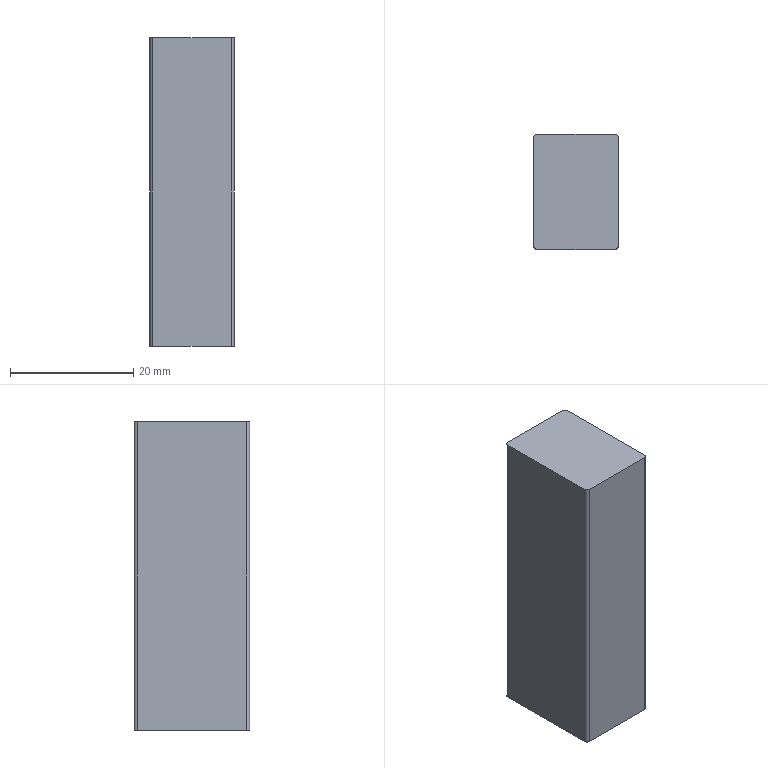Part | NX | features BREP 1 | 1 solid | 10 faces | box 13.656 x 18.683 x 50 mm | volume 12746 mm3 | plane 6 | cylinder 4 | commonest cylinder face diameters 1 x4
STEP:
#1=CARTESIAN_POINT('',(-6.328,9.342,-40.6));
#2=VERTEX_POINT('',#1);
#3=CARTESIAN_POINT('',(-6.828,8.842,-40.6));
#4=VERTEX_POINT('',#3);
#5=CARTESIAN_POINT('',(-6.328,8.842,-40.6));
#6=DIRECTION('',(0.,0.,1.));
#7=DIRECTION('',(1.,0.,0.));
#8=AXIS2_PLACEMENT_3D('',#5,#6,#7);
#9=CIRCLE('',#8,0.5);
#10=EDGE_CURVE('',#2,#4,#9,.T.);
#11=ORIENTED_EDGE('',*,*,#10,.F.);
#12=CARTESIAN_POINT('',(-6.328,9.342,-90.6));
#13=VERTEX_POINT('',#12);
#14=CARTESIAN_POINT('',(-6.328,9.342,-90.6));
#15=DIRECTION('',(0.,0.,1.));
#16=VECTOR('',#15,1000.);
#17=LINE('',#14,#16);
#18=EDGE_CURVE('',#13,#2,#17,.T.);
#19=ORIENTED_EDGE('',*,*,#18,.F.);
#20=CARTESIAN_POINT('',(-6.828,8.842,-90.6));
#21=VERTEX_POINT('',#20);
#22=CARTESIAN_POINT('',(-6.328,8.842,-90.6));
#23=DIRECTION('',(0.,0.,1.));
#24=DIRECTION('',(1.,0.,0.));
#25=AXIS2_PLACEMENT_3D('',#22,#23,#24);
#26=CIRCLE('',#25,0.5);
#27=EDGE_CURVE('',#13,#21,#26,.T.);
#28=ORIENTED_EDGE('',*,*,#27,.T.);
#29=CARTESIAN_POINT('',(-6.828,8.842,-90.6));
#30=DIRECTION('',(0.,0.,1.));
#31=VECTOR('',#30,1000.);
#32=LINE('',#29,#31);
#33=EDGE_CURVE('',#21,#4,#32,.T.);
#34=ORIENTED_EDGE('',*,*,#33,.T.);
#35=EDGE_LOOP('',(#11,#19,#28,#34));
#36=FACE_BOUND('',#35,.T.);
#37=CARTESIAN_POINT('',(-6.328,8.842,-90.6));
#38=DIRECTION('',(0.,0.,1.));
#39=DIRECTION('',(-1.,0.,0.));
#40=AXIS2_PLACEMENT_3D('',#37,#38,#39);
#41=CYLINDRICAL_SURFACE('',#40,0.5);
#42=ADVANCED_FACE('',(#36),#41,.T.);
#43=CARTESIAN_POINT('',(-6.828,-8.842,-40.6));
#44=VERTEX_POINT('',#43);
#45=CARTESIAN_POINT('',(-6.828,-8.842,-40.6));
#46=DIRECTION('',(0.,1.,0.));
#47=VECTOR('',#46,1000.);
#48=LINE('',#45,#47);
#49=EDGE_CURVE('',#44,#4,#48,.T.);
#50=ORIENTED_EDGE('',*,*,#49,.T.);
#51=ORIENTED_EDGE('',*,*,#33,.F.);
#52=CARTESIAN_POINT('',(-6.828,-8.842,-90.6));
#53=VERTEX_POINT('',#52);
#54=CARTESIAN_POINT('',(-6.828,-8.842,-90.6));
#55=DIRECTION('',(0.,1.,0.));
#56=VECTOR('',#55,1000.);
#57=LINE('',#54,#56);
#58=EDGE_CURVE('',#53,#21,#57,.T.);
#59=ORIENTED_EDGE('',*,*,#58,.F.);
#60=CARTESIAN_POINT('',(-6.828,-8.842,-90.6));
#61=DIRECTION('',(0.,0.,1.));
#62=VECTOR('',#61,1000.);
#63=LINE('',#60,#62);
#64=EDGE_CURVE('',#53,#44,#63,.T.);
#65=ORIENTED_EDGE('',*,*,#64,.T.);
#66=EDGE_LOOP('',(#50,#51,#59,#65));
#67=FACE_BOUND('',#66,.T.);
#68=CARTESIAN_POINT('',(-6.828,-8.842,-90.6));
#69=DIRECTION('',(1.,0.,0.));
#70=DIRECTION('',(0.,-1.,0.));
#71=AXIS2_PLACEMENT_3D('',#68,#69,#70);
#72=PLANE('',#71);
#73=ADVANCED_FACE('',(#67),#72,.F.);
#74=CARTESIAN_POINT('',(-6.328,-9.342,-40.6));
#75=VERTEX_POINT('',#74);
#76=CARTESIAN_POINT('',(-6.328,-8.842,-40.6));
#77=DIRECTION('',(0.,0.,1.));
#78=DIRECTION('',(1.,0.,0.));
#79=AXIS2_PLACEMENT_3D('',#76,#77,#78);
#80=CIRCLE('',#79,0.5);
#81=EDGE_CURVE('',#44,#75,#80,.T.);
#82=ORIENTED_EDGE('',*,*,#81,.F.);
#83=ORIENTED_EDGE('',*,*,#64,.F.);
#84=CARTESIAN_POINT('',(-6.328,-9.342,-90.6));
#85=VERTEX_POINT('',#84);
#86=CARTESIAN_POINT('',(-6.328,-8.842,-90.6));
#87=DIRECTION('',(0.,0.,1.));
#88=DIRECTION('',(1.,0.,0.));
#89=AXIS2_PLACEMENT_3D('',#86,#87,#88);
#90=CIRCLE('',#89,0.5);
#91=EDGE_CURVE('',#53,#85,#90,.T.);
#92=ORIENTED_EDGE('',*,*,#91,.T.);
#93=CARTESIAN_POINT('',(-6.328,-9.342,-90.6));
#94=DIRECTION('',(0.,0.,1.));
#95=VECTOR('',#94,1000.);
#96=LINE('',#93,#95);
#97=EDGE_CURVE('',#85,#75,#96,.T.);
#98=ORIENTED_EDGE('',*,*,#97,.T.);
#99=EDGE_LOOP('',(#82,#83,#92,#98));
#100=FACE_BOUND('',#99,.T.);
#101=CARTESIAN_POINT('',(-6.328,-8.842,-90.6));
#102=DIRECTION('',(0.,0.,1.));
#103=DIRECTION('',(-1.,0.,0.));
#104=AXIS2_PLACEMENT_3D('',#101,#102,#103);
#105=CYLINDRICAL_SURFACE('',#104,0.5);
#106=ADVANCED_FACE('',(#100),#105,.T.);
#107=CARTESIAN_POINT('',(6.328,-9.342,-40.6));
#108=VERTEX_POINT('',#107);
#109=CARTESIAN_POINT('',(6.328,-9.342,-40.6));
#110=DIRECTION('',(-1.,0.,0.));
#111=VECTOR('',#110,1000.);
#112=LINE('',#109,#111);
#113=EDGE_CURVE('',#108,#75,#112,.T.);
#114=ORIENTED_EDGE('',*,*,#113,.T.);
#115=ORIENTED_EDGE('',*,*,#97,.F.);
#116=CARTESIAN_POINT('',(6.328,-9.342,-90.6));
#117=VERTEX_POINT('',#116);
#118=CARTESIAN_POINT('',(6.328,-9.342,-90.6));
#119=DIRECTION('',(-1.,0.,0.));
#120=VECTOR('',#119,1000.);
#121=LINE('',#118,#120);
#122=EDGE_CURVE('',#117,#85,#121,.T.);
#123=ORIENTED_EDGE('',*,*,#122,.F.);
#124=CARTESIAN_POINT('',(6.328,-9.342,-90.6));
#125=DIRECTION('',(0.,0.,1.));
#126=VECTOR('',#125,1000.);
#127=LINE('',#124,#126);
#128=EDGE_CURVE('',#117,#108,#127,.T.);
#129=ORIENTED_EDGE('',*,*,#128,.T.);
#130=EDGE_LOOP('',(#114,#115,#123,#129));
#131=FACE_BOUND('',#130,.T.);
#132=CARTESIAN_POINT('',(6.328,-9.342,-90.6));
#133=DIRECTION('',(0.,1.,0.));
#134=DIRECTION('',(0.,0.,-1.));
#135=AXIS2_PLACEMENT_3D('',#132,#133,#134);
#136=PLANE('',#135);
#137=ADVANCED_FACE('',(#131),#136,.F.);
#138=CARTESIAN_POINT('',(6.828,-8.842,-40.6));
#139=VERTEX_POINT('',#138);
#140=CARTESIAN_POINT('',(6.328,-8.842,-40.6));
#141=DIRECTION('',(0.,0.,1.));
#142=DIRECTION('',(1.,0.,0.));
#143=AXIS2_PLACEMENT_3D('',#140,#141,#142);
#144=CIRCLE('',#143,0.5);
#145=EDGE_CURVE('',#108,#139,#144,.T.);
#146=ORIENTED_EDGE('',*,*,#145,.F.);
#147=ORIENTED_EDGE('',*,*,#128,.F.);
#148=CARTESIAN_POINT('',(6.828,-8.842,-90.6));
#149=VERTEX_POINT('',#148);
#150=CARTESIAN_POINT('',(6.328,-8.842,-90.6));
#151=DIRECTION('',(0.,0.,1.));
#152=DIRECTION('',(1.,0.,0.));
#153=AXIS2_PLACEMENT_3D('',#150,#151,#152);
#154=CIRCLE('',#153,0.5);
#155=EDGE_CURVE('',#117,#149,#154,.T.);
#156=ORIENTED_EDGE('',*,*,#155,.T.);
#157=CARTESIAN_POINT('',(6.828,-8.842,-90.6));
#158=DIRECTION('',(0.,0.,1.));
#159=VECTOR('',#158,1000.);
#160=LINE('',#157,#159);
#161=EDGE_CURVE('',#149,#139,#160,.T.);
#162=ORIENTED_EDGE('',*,*,#161,.T.);
#163=EDGE_LOOP('',(#146,#147,#156,#162));
#164=FACE_BOUND('',#163,.T.);
#165=CARTESIAN_POINT('',(6.328,-8.842,-90.6));
#166=DIRECTION('',(0.,0.,1.));
#167=DIRECTION('',(-1.,0.,0.));
#168=AXIS2_PLACEMENT_3D('',#165,#166,#167);
#169=CYLINDRICAL_SURFACE('',#168,0.5);
#170=ADVANCED_FACE('',(#164),#169,.T.);
#171=CARTESIAN_POINT('',(6.828,8.842,-40.6));
#172=VERTEX_POINT('',#171);
#173=CARTESIAN_POINT('',(6.828,8.842,-40.6));
#174=DIRECTION('',(0.,-1.,0.));
#175=VECTOR('',#174,1000.);
#176=LINE('',#173,#175);
#177=EDGE_CURVE('',#172,#139,#176,.T.);
#178=ORIENTED_EDGE('',*,*,#177,.T.);
#179=ORIENTED_EDGE('',*,*,#161,.F.);
#180=CARTESIAN_POINT('',(6.828,8.842,-90.6));
#181=VERTEX_POINT('',#180);
#182=CARTESIAN_POINT('',(6.828,8.842,-90.6));
#183=DIRECTION('',(0.,-1.,0.));
#184=VECTOR('',#183,1000.);
#185=LINE('',#182,#184);
#186=EDGE_CURVE('',#181,#149,#185,.T.);
#187=ORIENTED_EDGE('',*,*,#186,.F.);
#188=CARTESIAN_POINT('',(6.828,8.842,-90.6));
#189=DIRECTION('',(0.,0.,1.));
#190=VECTOR('',#189,1000.);
#191=LINE('',#188,#190);
#192=EDGE_CURVE('',#181,#172,#191,.T.);
#193=ORIENTED_EDGE('',*,*,#192,.T.);
#194=EDGE_LOOP('',(#178,#179,#187,#193));
#195=FACE_BOUND('',#194,.T.);
#196=CARTESIAN_POINT('',(6.828,8.842,-90.6));
#197=DIRECTION('',(-1.,0.,0.));
#198=DIRECTION('',(0.,0.,-1.));
#199=AXIS2_PLACEMENT_3D('',#196,#197,#198);
#200=PLANE('',#199);
#201=ADVANCED_FACE('',(#195),#200,.F.);
#202=CARTESIAN_POINT('',(6.328,9.342,-40.6));
#203=VERTEX_POINT('',#202);
#204=CARTESIAN_POINT('',(6.328,8.842,-40.6));
#205=DIRECTION('',(0.,0.,1.));
#206=DIRECTION('',(1.,0.,0.));
#207=AXIS2_PLACEMENT_3D('',#204,#205,#206);
#208=CIRCLE('',#207,0.5);
#209=EDGE_CURVE('',#172,#203,#208,.T.);
#210=ORIENTED_EDGE('',*,*,#209,.F.);
#211=ORIENTED_EDGE('',*,*,#192,.F.);
#212=CARTESIAN_POINT('',(6.328,9.342,-90.6));
#213=VERTEX_POINT('',#212);
#214=CARTESIAN_POINT('',(6.328,8.842,-90.6));
#215=DIRECTION('',(0.,0.,1.));
#216=DIRECTION('',(1.,0.,0.));
#217=AXIS2_PLACEMENT_3D('',#214,#215,#216);
#218=CIRCLE('',#217,0.5);
#219=EDGE_CURVE('',#181,#213,#218,.T.);
#220=ORIENTED_EDGE('',*,*,#219,.T.);
#221=CARTESIAN_POINT('',(6.328,9.342,-90.6));
#222=DIRECTION('',(0.,0.,1.));
#223=VECTOR('',#222,1000.);
#224=LINE('',#221,#223);
#225=EDGE_CURVE('',#213,#203,#224,.T.);
#226=ORIENTED_EDGE('',*,*,#225,.T.);
#227=EDGE_LOOP('',(#210,#211,#220,#226));
#228=FACE_BOUND('',#227,.T.);
#229=CARTESIAN_POINT('',(6.328,8.842,-90.6));
#230=DIRECTION('',(0.,0.,1.));
#231=DIRECTION('',(-1.,0.,0.));
#232=AXIS2_PLACEMENT_3D('',#229,#230,#231);
#233=CYLINDRICAL_SURFACE('',#232,0.5);
#234=ADVANCED_FACE('',(#228),#233,.T.);
#235=CARTESIAN_POINT('',(-6.328,9.342,-40.6));
#236=DIRECTION('',(1.,0.,0.));
#237=VECTOR('',#236,1000.);
#238=LINE('',#235,#237);
#239=EDGE_CURVE('',#2,#203,#238,.T.);
#240=ORIENTED_EDGE('',*,*,#239,.T.);
#241=ORIENTED_EDGE('',*,*,#225,.F.);
#242=CARTESIAN_POINT('',(-6.328,9.342,-90.6));
#243=DIRECTION('',(1.,0.,0.));
#244=VECTOR('',#243,1000.);
#245=LINE('',#242,#244);
#246=EDGE_CURVE('',#13,#213,#245,.T.);
#247=ORIENTED_EDGE('',*,*,#246,.F.);
#248=ORIENTED_EDGE('',*,*,#18,.T.);
#249=EDGE_LOOP('',(#240,#241,#247,#248));
#250=FACE_BOUND('',#249,.T.);
#251=CARTESIAN_POINT('',(-6.328,9.342,-90.6));
#252=DIRECTION('',(0.,-1.,0.));
#253=DIRECTION('',(-1.,0.,0.));
#254=AXIS2_PLACEMENT_3D('',#251,#252,#253);
#255=PLANE('',#254);
#256=ADVANCED_FACE('',(#250),#255,.F.);
#257=ORIENTED_EDGE('',*,*,#27,.F.);
#258=ORIENTED_EDGE('',*,*,#246,.T.);
#259=ORIENTED_EDGE('',*,*,#219,.F.);
#260=ORIENTED_EDGE('',*,*,#186,.T.);
#261=ORIENTED_EDGE('',*,*,#155,.F.);
#262=ORIENTED_EDGE('',*,*,#122,.T.);
#263=ORIENTED_EDGE('',*,*,#91,.F.);
#264=ORIENTED_EDGE('',*,*,#58,.T.);
#265=EDGE_LOOP('',(#257,#258,#259,#260,#261,#262,#263,#264));
#266=FACE_BOUND('',#265,.T.);
#267=CARTESIAN_POINT('',(-6.328,8.842,-90.6));
#268=DIRECTION('',(0.,0.,1.));
#269=DIRECTION('',(-1.,0.,0.));
#270=AXIS2_PLACEMENT_3D('',#267,#268,#269);
#271=PLANE('',#270);
#272=ADVANCED_FACE('',(#266),#271,.F.);
#273=ORIENTED_EDGE('',*,*,#10,.T.);
#274=ORIENTED_EDGE('',*,*,#49,.F.);
#275=ORIENTED_EDGE('',*,*,#81,.T.);
#276=ORIENTED_EDGE('',*,*,#113,.F.);
#277=ORIENTED_EDGE('',*,*,#145,.T.);
#278=ORIENTED_EDGE('',*,*,#177,.F.);
#279=ORIENTED_EDGE('',*,*,#209,.T.);
#280=ORIENTED_EDGE('',*,*,#239,.F.);
#281=EDGE_LOOP('',(#273,#274,#275,#276,#277,#278,#279,#280));
#282=FACE_BOUND('',#281,.T.);
#283=CARTESIAN_POINT('',(-6.328,8.842,-40.6));
#284=DIRECTION('',(0.,0.,1.));
#285=DIRECTION('',(-1.,0.,0.));
#286=AXIS2_PLACEMENT_3D('',#283,#284,#285);
#287=PLANE('',#286);
#288=ADVANCED_FACE('',(#282),#287,.T.);
#289=CLOSED_SHELL('',(#42,#73,#106,#137,#170,#201,#234,#256,#272,#288));
#290=MANIFOLD_SOLID_BREP('',#289);
#291=(LENGTH_UNIT()NAMED_UNIT(*)SI_UNIT(.MILLI.,.METRE.));
#292=UNCERTAINTY_MEASURE_WITH_UNIT(LENGTH_MEASURE(0.00001),#291,'','');
#293=(NAMED_UNIT(*)PLANE_ANGLE_UNIT()SI_UNIT($,.RADIAN.));
#294=(NAMED_UNIT(*)SI_UNIT($,.STERADIAN.)SOLID_ANGLE_UNIT());
#295=(GEOMETRIC_REPRESENTATION_CONTEXT(3)GLOBAL_UNCERTAINTY_ASSIGNED_CONTEXT((#292))GLOBAL_UNIT_ASSIGNED_CONTEXT((#291,#293,#294))REPRESENTATION_CONTEXT('',''));
#296=ADVANCED_BREP_SHAPE_REPRESENTATION('',(#290),#295);